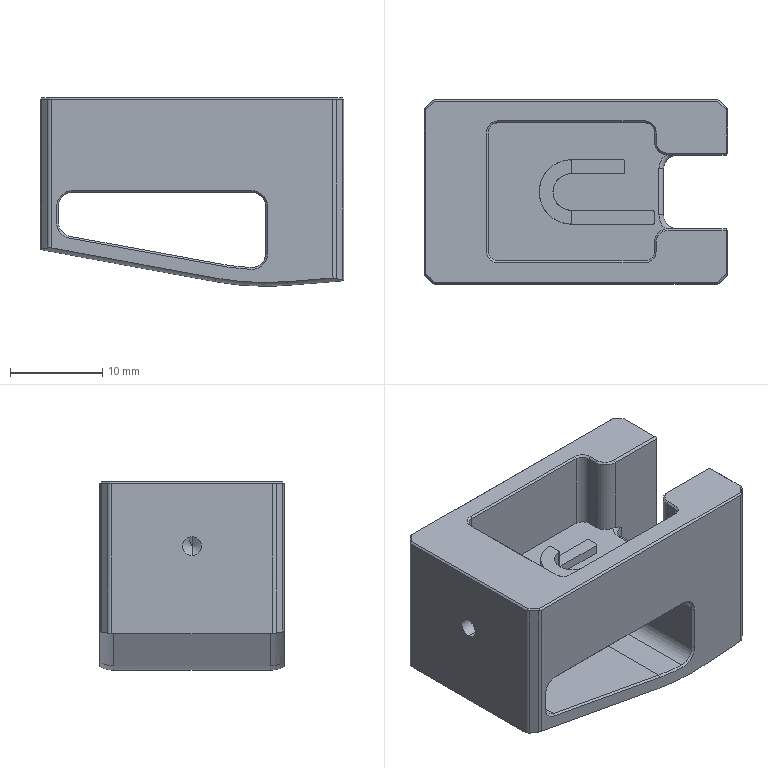NC program | NX | posted with a generic post | part box 33 x 20 x 20.478 mm
Lines 5322 to 6458 of 8500:
(CAVITY_MILL_COPY_COPY , TOOL : D2)
N10606 T17 M6
N10608 G54
N10610 G17 G0 G90 X-6.603 Y6.151 B0. C0. S9500 M3
N10612 G43 Z11. H17
N10614 Z1.351
N10616 G94 G1 Z-0.149 F1000.
N10618 G3 X-7.403 Y6.551 R1.
N10620 G1 X-8.5
N10622 X-8.554 Y6.554
N10624 X-8.551 Y6.5
N10626 Y5.403
N10628 G3 X-8.151 Y4.603 R1.
N10630 G1 Z1.351
N10632 G0 Z11.
N10634 X-6.552 Y6.1
N10636 Z1.203
N10638 G1 Z-0.297
N10640 G3 X-7.352 Y6.5 R1.
N10642 G1 X-8.5
N10644 Y5.352
N10646 G3 X-8.1 Y4.552 R1.
N10648 G1 Z1.203
N10650 G0 Z11.
N10652 X-6.552 Y6.1
N10654 Z1.054
N10656 G1 Z-0.446
N10658 G3 X-7.352 Y6.5 R1.
N10660 G1 X-8.5
N10662 Y5.352
N10664 G3 X-8.1 Y4.552 R1.
N10666 G1 Z1.054
N10668 G0 Z11.
N10670 X-6.552 Y6.1
N10672 Z0.905
N10674 G1 Z-0.595
N10676 G3 X-7.352 Y6.5 R1.
N10678 G1 X-8.5
N10680 Y5.352
N10682 G3 X-8.1 Y4.552 R1.
N10684 G1 Z0.905
N10686 G0 Z11.
N10688 X-6.552 Y6.1
N10690 Z0.756
N10692 G1 Z-0.744
N10694 G3 X-7.352 Y6.5 R1.
N10696 G1 X-8.5
N10698 Y5.352
N10700 G3 X-8.1 Y4.552 R1.
N10702 G1 Z0.756
N10704 G0 Z11.
N10706 X-6.552 Y6.1
N10708 Z0.608
N10710 G1 Z-0.892
N10712 G3 X-7.352 Y6.5 R1.
N10714 G1 X-8.5
N10716 Y5.352
N10718 G3 X-8.1 Y4.552 R1.
N10720 G1 Z0.608
N10722 G0 Z11.
N10724 X-6.552 Y6.1
N10726 Z0.459
N10728 G1 Z-1.041
N10730 G3 X-7.352 Y6.5 R1.
N10732 G1 X-8.5
N10734 Y5.352
N10736 G3 X-8.1 Y4.552 R1.
N10738 G1 Z0.459
N10740 G0 Z11.
N10742 X-6.552 Y6.1
N10744 Z0.31
N10746 G1 Z-1.19
N10748 G3 X-7.352 Y6.5 R1.
N10750 G1 X-8.5
N10752 Y5.352
N10754 G3 X-8.1 Y4.552 R1.
N10756 G1 Z0.31
N10758 G0 Z11.
N10760 X-6.552 Y6.1
N10762 Z0.162
N10764 G1 Z-1.338
N10766 G3 X-7.352 Y6.5 R1.
N10768 G1 X-8.5
N10770 Y5.352
N10772 G3 X-8.1 Y4.552 R1.
N10774 G1 Z0.162
N10776 G0 Z11.
N10778 X-6.552 Y6.1
N10780 Z0.013
N10782 G1 Z-1.487
N10784 G3 X-7.352 Y6.5 R1.
N10786 G1 X-8.5
N10788 Y5.352
N10790 G3 X-8.1 Y4.552 R1.
N10792 G1 Z0.013
N10794 G0 X-6.552 Y6.1 Z-0.136
N10796 G1 Z-1.636
N10798 G3 X-7.352 Y6.5 R1.
N10800 G1 X-8.5
N10802 Y5.352
N10804 G3 X-8.1 Y4.552 R1.
N10806 G1 Z-0.136
N10808 G0 X-6.552 Y6.1 Z-0.285
N10810 G1 Z-1.785
N10812 G3 X-7.352 Y6.5 R1.
N10814 G1 X-8.5
N10816 Y5.352
N10818 G3 X-8.1 Y4.552 R1.
N10820 G1 Z-0.285
N10822 G0 X-6.552 Y6.1 Z-0.433
N10824 G1 Z-1.933
N10826 G3 X-7.352 Y6.5 R1.
N10828 G1 X-8.5
N10830 Y5.352
N10832 G3 X-8.1 Y4.552 R1.
N10834 G1 Z-0.433
N10836 G0 X-6.552 Y6.1 Z-0.582
N10838 G1 Z-2.082
N10840 G3 X-7.352 Y6.5 R1.
N10842 G1 X-8.5
N10844 Y5.352
N10846 G3 X-8.1 Y4.552 R1.
N10848 G1 Z-0.582
N10850 G0 X-6.552 Y6.1 Z-0.731
N10852 G1 Z-2.231
N10854 G3 X-7.352 Y6.5 R1.
N10856 G1 X-8.5
N10858 Y5.352
N10860 G3 X-8.1 Y4.552 R1.
N10862 G1 Z-0.731
N10864 G0 X-6.552 Y6.1 Z-0.879
N10866 G1 Z-2.379
N10868 G3 X-7.352 Y6.5 R1.
N10870 G1 X-8.5
N10872 Y5.352
N10874 G3 X-8.1 Y4.552 R1.
N10876 G1 Z-0.879
N10878 G0 X-6.552 Y6.1 Z-1.028
N10880 G1 Z-2.528
N10882 G3 X-7.352 Y6.5 R1.
N10884 G1 X-8.5
N10886 Y5.352
N10888 G3 X-8.1 Y4.552 R1.
N10890 G1 Z-1.028
N10892 G0 X-6.552 Y6.1 Z-1.177
N10894 G1 Z-2.677
N10896 G3 X-7.352 Y6.5 R1.
N10898 G1 X-8.5
N10900 Y5.352
N10902 G3 X-8.1 Y4.552 R1.
N10904 G1 Z-1.177
N10906 G0 X-6.552 Y6.1 Z-1.326
N10908 G1 Z-2.826
N10910 G3 X-7.352 Y6.5 R1.
N10912 G1 X-8.5
N10914 Y5.352
N10916 G3 X-8.1 Y4.552 R1.
N10918 G1 Z-1.326
N10920 G0 X-6.552 Y6.1 Z-1.474
N10922 G1 Z-2.974
N10924 G3 X-7.352 Y6.5 R1.
N10926 G1 X-8.5
N10928 Y5.352
N10930 G3 X-8.1 Y4.552 R1.
N10932 G1 Z-1.474
N10934 G0 X-6.552 Y6.1 Z-1.623
N10936 G1 Z-3.123
N10938 G3 X-7.352 Y6.5 R1.
N10940 G1 X-8.5
N10942 Y5.352
N10944 G3 X-8.1 Y4.552 R1.
N10946 G1 Z-1.623
N10948 G0 X-6.552 Y6.1 Z-1.772
N10950 G1 Z-3.272
N10952 G3 X-7.352 Y6.5 R1.
N10954 G1 X-8.5
N10956 Y5.352
N10958 G3 X-8.1 Y4.552 R1.
N10960 G1 Z-1.772
N10962 G0 X-6.552 Y6.1 Z-1.921
N10964 G1 Z-3.421
N10966 G3 X-7.352 Y6.5 R1.
N10968 G1 X-8.5
N10970 Y5.352
N10972 G3 X-8.1 Y4.552 R1.
N10974 G1 Z-1.921
N10976 G0 X-6.552 Y6.1 Z-2.069
N10978 G1 Z-3.569
N10980 G3 X-7.352 Y6.5 R1.
N10982 G1 X-8.5
N10984 Y5.352
N10986 G3 X-8.1 Y4.552 R1.
N10988 G1 Z-2.069
N10990 G0 X-6.552 Y6.1 Z-2.218
N10992 G1 Z-3.718
N10994 G3 X-7.352 Y6.5 R1.
N10996 G1 X-8.5
N10998 Y5.352
N11000 G3 X-8.1 Y4.552 R1.
N11002 G1 Z-2.218
N11004 G0 X-6.552 Y6.1 Z-2.367
N11006 G1 Z-3.867
N11008 G3 X-7.352 Y6.5 R1.
N11010 G1 X-8.5
N11012 Y5.352
N11014 G3 X-8.1 Y4.552 R1.
N11016 G1 Z-2.367
N11018 G0 X-6.552 Y6.1 Z-2.515
N11020 G1 Z-4.015
N11022 G3 X-7.352 Y6.5 R1.
N11024 G1 X-8.5
N11026 Y5.352
N11028 G3 X-8.1 Y4.552 R1.
N11030 G1 Z-2.515
N11032 G0 X-6.552 Y6.1 Z-2.664
N11034 G1 Z-4.164
N11036 G3 X-7.352 Y6.5 R1.
N11038 G1 X-8.5
N11040 Y5.352
N11042 G3 X-8.1 Y4.552 R1.
N11044 G1 Z-2.664
N11046 G0 X-6.552 Y6.1 Z-2.813
N11048 G1 Z-4.313
N11050 G3 X-7.352 Y6.5 R1.
N11052 G1 X-8.5
N11054 Y5.352
N11056 G3 X-8.1 Y4.552 R1.
N11058 G1 Z-2.813
N11060 G0 X-6.552 Y6.1 Z-2.962
N11062 G1 Z-4.462
N11064 G3 X-7.352 Y6.5 R1.
N11066 G1 X-8.5
N11068 Y5.352
N11070 G3 X-8.1 Y4.552 R1.
N11072 G1 Z-2.962
N11074 G0 X-6.552 Y6.1 Z-3.11
N11076 G1 Z-4.61
N11078 G3 X-7.352 Y6.5 R1.
N11080 G1 X-8.5
N11082 Y5.352
N11084 G3 X-8.1 Y4.552 R1.
N11086 G1 Z-3.11
N11088 G0 X-6.552 Y6.1 Z-3.259
N11090 G1 Z-4.759
N11092 G3 X-7.352 Y6.5 R1.
N11094 G1 X-8.5
N11096 Y5.352
N11098 G3 X-8.1 Y4.552 R1.
N11100 G1 Z-3.259
N11102 G0 X-6.552 Y6.1 Z-3.408
N11104 G1 Z-4.908
N11106 G3 X-7.352 Y6.5 R1.
N11108 G1 X-8.5
N11110 Y5.352
N11112 G3 X-8.1 Y4.552 R1.
N11114 G1 Z-3.408
N11116 G0 X-6.552 Y6.1 Z-3.556
N11118 G1 Z-5.056
N11120 G3 X-7.352 Y6.5 R1.
N11122 G1 X-8.5
N11124 Y5.352
N11126 G3 X-8.1 Y4.552 R1.
N11128 G1 Z-3.556
N11130 G0 X-6.552 Y6.1 Z-3.705
N11132 G1 Z-5.205
N11134 G3 X-7.352 Y6.5 R1.
N11136 G1 X-8.5
N11138 Y5.352
N11140 G3 X-8.1 Y4.552 R1.
N11142 G1 Z-3.705
N11144 G0 X-6.552 Y6.1 Z-3.854
N11146 G1 Z-5.354
N11148 G3 X-7.352 Y6.5 R1.
N11150 G1 X-8.5
N11152 Y5.352
N11154 G3 X-8.1 Y4.552 R1.
N11156 G1 Z-3.854
N11158 G0 X-6.552 Y6.1 Z-4.003
N11160 G1 Z-5.503
N11162 G3 X-7.352 Y6.5 R1.
N11164 G1 X-8.5
N11166 Y5.352
N11168 G3 X-8.1 Y4.552 R1.
N11170 G1 Z-4.003
N11172 G0 X-6.552 Y6.1 Z-4.151
N11174 G1 Z-5.651
N11176 G3 X-7.352 Y6.5 R1.
N11178 G1 X-8.5
N11180 Y5.352
N11182 G3 X-8.1 Y4.552 R1.
N11184 G1 Z-4.151
N11186 G0 X-6.552 Y6.1 Z-4.3
N11188 G1 Z-5.8
N11190 G3 X-7.352 Y6.5 R1.
N11192 G1 X-8.5
N11194 Y5.352
N11196 G3 X-8.1 Y4.552 R1.
N11198 G1 Z-4.3
N11200 G0 X-6.552 Y6.1 Z-4.443
N11202 G1 Z-5.943
N11204 G3 X-7.352 Y6.5 R1.
N11206 G1 X-8.5
N11208 Y5.352
N11210 G3 X-8.1 Y4.552 R1.
N11212 G1 Z-4.443
N11214 G0 X-6.552 Y6.1 Z-4.586
N11216 G1 Z-6.086
N11218 G3 X-7.352 Y6.5 R1.
N11220 G1 X-8.5
N11222 Y5.352
N11224 G3 X-8.1 Y4.552 R1.
N11226 G1 Z-4.586
N11228 G0 X-6.552 Y6.1 Z-4.729
N11230 G1 Z-6.229
N11232 G3 X-7.352 Y6.5 R1.
N11234 G1 X-8.5
N11236 Y5.352
N11238 G3 X-8.1 Y4.552 R1.
N11240 G1 Z-4.729
N11242 G0 X-6.552 Y6.1 Z-4.871
N11244 G1 Z-6.371
N11246 G3 X-7.352 Y6.5 R1.
N11248 G1 X-8.5
N11250 Y5.352
N11252 G3 X-8.1 Y4.552 R1.
N11254 G1 Z-4.871
N11256 G0 X-6.552 Y6.1 Z-5.014
N11258 G1 Z-6.514
N11260 G3 X-7.352 Y6.5 R1.
N11262 G1 X-8.5
N11264 Y5.352
N11266 G3 X-8.1 Y4.552 R1.
N11268 G1 Z-5.014
N11270 G0 X-6.552 Y6.1 Z-5.157
N11272 G1 Z-6.657
N11274 G3 X-7.352 Y6.5 R1.
N11276 G1 X-8.5
N11278 Y5.352
N11280 G3 X-8.1 Y4.552 R1.
N11282 G1 Z-5.157
N11284 G0 X-6.552 Y6.1 Z-5.3
N11286 G1 Z-6.8
N11288 G3 X-7.352 Y6.5 R1.
N11290 G1 X-8.5
N11292 Y5.352
N11294 G3 X-8.1 Y4.552 R1.
N11296 G1 Z-5.3
N11298 G0 X-6.552 Y6.1 Z-5.443
N11300 G1 Z-6.943
N11302 G3 X-7.352 Y6.5 R1.
N11304 G1 X-8.5
N11306 Y5.352
N11308 G3 X-8.1 Y4.552 R1.
N11310 G1 Z-5.443
N11312 G0 X-6.552 Y6.1 Z-5.586
N11314 G1 Z-7.086
N11316 G3 X-7.352 Y6.5 R1.
N11318 G1 X-8.5
N11320 Y5.352
N11322 G3 X-8.1 Y4.552 R1.
N11324 G1 Z-5.586
N11326 G0 X-6.552 Y6.1 Z-5.729
N11328 G1 Z-7.229
N11330 G3 X-7.352 Y6.5 R1.
N11332 G1 X-8.5
N11334 Y5.352
N11336 G3 X-8.1 Y4.552 R1.
N11338 G1 Z-5.729
N11340 G0 X-6.552 Y6.1 Z-5.871
N11342 G1 Z-7.371
N11344 G3 X-7.352 Y6.5 R1.
N11346 G1 X-8.5
N11348 Y5.352
N11350 G3 X-8.1 Y4.552 R1.
N11352 G1 Z-5.871
N11354 G0 X-6.552 Y6.1 Z-6.014
N11356 G1 Z-7.514
N11358 G3 X-7.352 Y6.5 R1.
N11360 G1 X-8.5
N11362 Y5.352
N11364 G3 X-8.1 Y4.552 R1.
N11366 G1 Z-6.014
N11368 G0 X-6.552 Y6.1 Z-6.157
N11370 G1 Z-7.657
N11372 G3 X-7.352 Y6.5 R1.
N11374 G1 X-8.5
N11376 Y5.352
N11378 G3 X-8.1 Y4.552 R1.
N11380 G1 Z-6.157
N11382 G0 X-6.552 Y6.1 Z-6.3
N11384 G1 Z-7.8
N11386 G3 X-7.352 Y6.5 R1.
N11388 G1 X-8.5
N11390 Y5.352
N11392 G3 X-8.1 Y4.552 R1.
N11394 G1 Z-6.3
N11396 G0 X-6.552 Y6.1 Z-6.443
N11398 G1 Z-7.943
N11400 G3 X-7.352 Y6.5 R1.
N11402 G1 X-8.5
N11404 Y5.352
N11406 G3 X-8.1 Y4.552 R1.
N11408 G1 Z-6.443
N11410 G0 X-6.552 Y6.1 Z-6.586
N11412 G1 Z-8.086
N11414 G3 X-7.352 Y6.5 R1.
N11416 G1 X-8.5
N11418 Y5.352
N11420 G3 X-8.1 Y4.552 R1.
N11422 G1 Z-6.586
N11424 G0 X-6.552 Y6.1 Z-6.729
N11426 G1 Z-8.229
N11428 G3 X-7.352 Y6.5 R1.
N11430 G1 X-8.5
N11432 Y5.352
N11434 G3 X-8.1 Y4.552 R1.
N11436 G1 Z-6.729
N11438 G0 X-6.552 Y6.1 Z-6.871
N11440 G1 Z-8.371
N11442 G3 X-7.352 Y6.5 R1.
N11444 G1 X-8.5
N11446 Y5.352
N11448 G3 X-8.1 Y4.552 R1.
N11450 G1 Z-6.871
N11452 G0 X-6.552 Y6.1 Z-7.014
N11454 G1 Z-8.514
N11456 G3 X-7.352 Y6.5 R1.
N11458 G1 X-8.5
N11460 Y5.352
N11462 G3 X-8.1 Y4.552 R1.
N11464 G1 Z-7.014
N11466 G0 X-6.552 Y6.1 Z-7.157
N11468 G1 Z-8.657
N11470 G3 X-7.352 Y6.5 R1.
N11472 G1 X-8.5
N11474 Y5.352
N11476 G3 X-8.1 Y4.552 R1.
N11478 G1 Z-7.157
N11480 G0 X-6.552 Y6.1 Z-7.3
N11482 G1 Z-8.8
N11484 G3 X-7.352 Y6.5 R1.
N11486 G1 X-8.5
N11488 Y5.352
N11490 G3 X-8.1 Y4.552 R1.
N11492 G1 Z-7.3
N11494 G0 Z11.
N11496 X-8.151 Y-4.603
N11498 Z1.351
N11500 G1 Z-0.149
N11502 G3 X-8.551 Y-5.403 R1.
N11504 G1 Y-6.5
N11506 X-8.554 Y-6.554
N11508 X-8.5 Y-6.551
N11510 X-7.403
N11512 G3 X-6.603 Y-6.151 R1.
N11514 G1 Z1.351
N11516 G0 Z11.
N11518 X-8.1 Y-4.552
N11520 Z1.203
N11522 G1 Z-0.297
N11524 G3 X-8.5 Y-5.352 R1.
N11526 G1 Y-6.5
N11528 X-7.352
N11530 G3 X-6.552 Y-6.1 R1.
N11532 G1 Z1.203
N11534 G0 Z11.
N11536 X-8.1 Y-4.552
N11538 Z1.054
N11540 G1 Z-0.446
N11542 G3 X-8.5 Y-5.352 R1.
N11544 G1 Y-6.5
N11546 X-7.352
N11548 G3 X-6.552 Y-6.1 R1.
N11550 G1 Z1.054
N11552 G0 Z11.
N11554 X-8.1 Y-4.552
N11556 Z0.905
N11558 G1 Z-0.595
N11560 G3 X-8.5 Y-5.352 R1.
N11562 G1 Y-6.5
N11564 X-7.352
N11566 G3 X-6.552 Y-6.1 R1.
N11568 G1 Z0.905
N11570 G0 Z11.
N11572 X-8.1 Y-4.552
N11574 Z0.756
N11576 G1 Z-0.744
N11578 G3 X-8.5 Y-5.352 R1.
N11580 G1 Y-6.5
N11582 X-7.352
N11584 G3 X-6.552 Y-6.1 R1.
N11586 G1 Z0.756
N11588 G0 Z11.
N11590 X-8.1 Y-4.552
N11592 Z0.608
N11594 G1 Z-0.892
N11596 G3 X-8.5 Y-5.352 R1.
N11598 G1 Y-6.5
N11600 X-7.352
N11602 G3 X-6.552 Y-6.1 R1.
N11604 G1 Z0.608
N11606 G0 Z11.
N11608 X-8.1 Y-4.552
N11610 Z0.459
N11612 G1 Z-1.041
N11614 G3 X-8.5 Y-5.352 R1.
N11616 G1 Y-6.5
N11618 X-7.352
N11620 G3 X-6.552 Y-6.1 R1.
N11622 G1 Z0.459
N11624 G0 Z11.
N11626 X-8.1 Y-4.552
N11628 Z0.31
N11630 G1 Z-1.19
N11632 G3 X-8.5 Y-5.352 R1.
N11634 G1 Y-6.5
N11636 X-7.352
N11638 G3 X-6.552 Y-6.1 R1.
N11640 G1 Z0.31
N11642 G0 Z11.
N11644 X-8.1 Y-4.552
N11646 Z0.162
N11648 G1 Z-1.338
N11650 G3 X-8.5 Y-5.352 R1.
N11652 G1 Y-6.5
N11654 X-7.352
N11656 G3 X-6.552 Y-6.1 R1.
N11658 G1 Z0.162
N11660 G0 Z11.
N11662 X-8.1 Y-4.552
N11664 Z0.013
N11666 G1 Z-1.487
N11668 G3 X-8.5 Y-5.352 R1.
N11670 G1 Y-6.5
N11672 X-7.352
N11674 G3 X-6.552 Y-6.1 R1.
N11676 G1 Z0.013
N11678 G0 X-8.1 Y-4.552 Z-0.136
N11680 G1 Z-1.636
N11682 G3 X-8.5 Y-5.352 R1.
N11684 G1 Y-6.5
N11686 X-7.352
N11688 G3 X-6.552 Y-6.1 R1.
N11690 G1 Z-0.136
N11692 G0 X-8.1 Y-4.552 Z-0.285
N11694 G1 Z-1.785
N11696 G3 X-8.5 Y-5.352 R1.
N11698 G1 Y-6.5
N11700 X-7.352
N11702 G3 X-6.552 Y-6.1 R1.
N11704 G1 Z-0.285
N11706 G0 X-8.1 Y-4.552 Z-0.433
N11708 G1 Z-1.933
N11710 G3 X-8.5 Y-5.352 R1.
N11712 G1 Y-6.5
N11714 X-7.352
N11716 G3 X-6.552 Y-6.1 R1.
N11718 G1 Z-0.433
N11720 G0 X-8.1 Y-4.552 Z-0.582
N11722 G1 Z-2.082
N11724 G3 X-8.5 Y-5.352 R1.
N11726 G1 Y-6.5
N11728 X-7.352
N11730 G3 X-6.552 Y-6.1 R1.
N11732 G1 Z-0.582
N11734 G0 X-8.1 Y-4.552 Z-0.731
N11736 G1 Z-2.231
N11738 G3 X-8.5 Y-5.352 R1.
N11740 G1 Y-6.5
N11742 X-7.352
N11744 G3 X-6.552 Y-6.1 R1.
N11746 G1 Z-0.731
N11748 G0 X-8.1 Y-4.552 Z-0.879
N11750 G1 Z-2.379
N11752 G3 X-8.5 Y-5.352 R1.
N11754 G1 Y-6.5
N11756 X-7.352
N11758 G3 X-6.552 Y-6.1 R1.
N11760 G1 Z-0.879
N11762 G0 X-8.1 Y-4.552 Z-1.028
N11764 G1 Z-2.528
N11766 G3 X-8.5 Y-5.352 R1.
N11768 G1 Y-6.5
N11770 X-7.352
N11772 G3 X-6.552 Y-6.1 R1.
N11774 G1 Z-1.028
N11776 G0 X-8.1 Y-4.552 Z-1.177
N11778 G1 Z-2.677
N11780 G3 X-8.5 Y-5.352 R1.
N11782 G1 Y-6.5
N11784 X-7.352
N11786 G3 X-6.552 Y-6.1 R1.
N11788 G1 Z-1.177
N11790 G0 X-8.1 Y-4.552 Z-1.326
N11792 G1 Z-2.826
N11794 G3 X-8.5 Y-5.352 R1.
N11796 G1 Y-6.5
N11798 X-7.352
N11800 G3 X-6.552 Y-6.1 R1.
N11802 G1 Z-1.326
N11804 G0 X-8.1 Y-4.552 Z-1.474
N11806 G1 Z-2.974
N11808 G3 X-8.5 Y-5.352 R1.
N11810 G1 Y-6.5
N11812 X-7.352
N11814 G3 X-6.552 Y-6.1 R1.
N11816 G1 Z-1.474
N11818 G0 X-8.1 Y-4.552 Z-1.623
N11820 G1 Z-3.123
N11822 G3 X-8.5 Y-5.352 R1.
N11824 G1 Y-6.5
N11826 X-7.352
N11828 G3 X-6.552 Y-6.1 R1.
N11830 G1 Z-1.623
N11832 G0 X-8.1 Y-4.552 Z-1.772
N11834 G1 Z-3.272
N11836 G3 X-8.5 Y-5.352 R1.
N11838 G1 Y-6.5
N11840 X-7.352
N11842 G3 X-6.552 Y-6.1 R1.
N11844 G1 Z-1.772
N11846 G0 X-8.1 Y-4.552 Z-1.921
N11848 G1 Z-3.421
N11850 G3 X-8.5 Y-5.352 R1.
N11852 G1 Y-6.5
N11854 X-7.352
N11856 G3 X-6.552 Y-6.1 R1.
N11858 G1 Z-1.921
N11860 G0 X-8.1 Y-4.552 Z-2.069
N11862 G1 Z-3.569
N11864 G3 X-8.5 Y-5.352 R1.
N11866 G1 Y-6.5
N11868 X-7.352
N11870 G3 X-6.552 Y-6.1 R1.
N11872 G1 Z-2.069
N11874 G0 X-8.1 Y-4.552 Z-2.218
N11876 G1 Z-3.718
N11878 G3 X-8.5 Y-5.352 R1.
N11880 G1 Y-6.5
N11882 X-7.352
N11884 G3 X-6.552 Y-6.1 R1.
N11886 G1 Z-2.218
N11888 G0 X-8.1 Y-4.552 Z-2.367
N11890 G1 Z-3.867
N11892 G3 X-8.5 Y-5.352 R1.
N11894 G1 Y-6.5
N11896 X-7.352
N11898 G3 X-6.552 Y-6.1 R1.
N11900 G1 Z-2.367
N11902 G0 X-8.1 Y-4.552 Z-2.515
N11904 G1 Z-4.015
N11906 G3 X-8.5 Y-5.352 R1.
N11908 G1 Y-6.5
N11910 X-7.352
N11912 G3 X-6.552 Y-6.1 R1.
N11914 G1 Z-2.515
N11916 G0 X-8.1 Y-4.552 Z-2.664
N11918 G1 Z-4.164
N11920 G3 X-8.5 Y-5.352 R1.
N11922 G1 Y-6.5
N11924 X-7.352
N11926 G3 X-6.552 Y-6.1 R1.
N11928 G1 Z-2.664
N11930 G0 X-8.1 Y-4.552 Z-2.813
N11932 G1 Z-4.313
N11934 G3 X-8.5 Y-5.352 R1.
N11936 G1 Y-6.5
N11938 X-7.352
N11940 G3 X-6.552 Y-6.1 R1.
N11942 G1 Z-2.813
N11944 G0 X-8.1 Y-4.552 Z-2.962
N11946 G1 Z-4.462
N11948 G3 X-8.5 Y-5.352 R1.
N11950 G1 Y-6.5
N11952 X-7.352
N11954 G3 X-6.552 Y-6.1 R1.
N11956 G1 Z-2.962
N11958 G0 X-8.1 Y-4.552 Z-3.11
N11960 G1 Z-4.61
N11962 G3 X-8.5 Y-5.352 R1.
N11964 G1 Y-6.5
N11966 X-7.352
N11968 G3 X-6.552 Y-6.1 R1.
N11970 G1 Z-3.11
N11972 G0 X-8.1 Y-4.552 Z-3.259
N11974 G1 Z-4.759
N11976 G3 X-8.5 Y-5.352 R1.
N11978 G1 Y-6.5
N11980 X-7.352
N11982 G3 X-6.552 Y-6.1 R1.
N11984 G1 Z-3.259
N11986 G0 X-8.1 Y-4.552 Z-3.408
N11988 G1 Z-4.908
N11990 G3 X-8.5 Y-5.352 R1.
N11992 G1 Y-6.5
N11994 X-7.352
N11996 G3 X-6.552 Y-6.1 R1.
N11998 G1 Z-3.408
N12000 G0 X-8.1 Y-4.552 Z-3.556
N12002 G1 Z-5.056
N12004 G3 X-8.5 Y-5.352 R1.
N12006 G1 Y-6.5
N12008 X-7.352
N12010 G3 X-6.552 Y-6.1 R1.
N12012 G1 Z-3.556
N12014 G0 X-8.1 Y-4.552 Z-3.705
N12016 G1 Z-5.205
N12018 G3 X-8.5 Y-5.352 R1.
N12020 G1 Y-6.5
N12022 X-7.352
N12024 G3 X-6.552 Y-6.1 R1.
N12026 G1 Z-3.705
N12028 G0 X-8.1 Y-4.552 Z-3.854
N12030 G1 Z-5.354
N12032 G3 X-8.5 Y-5.352 R1.
N12034 G1 Y-6.5
N12036 X-7.352
N12038 G3 X-6.552 Y-6.1 R1.
N12040 G1 Z-3.854
N12042 G0 X-8.1 Y-4.552 Z-4.003
N12044 G1 Z-5.503
N12046 G3 X-8.5 Y-5.352 R1.
N12048 G1 Y-6.5
N12050 X-7.352
N12052 G3 X-6.552 Y-6.1 R1.
N12054 G1 Z-4.003
N12056 G0 X-8.1 Y-4.552 Z-4.151
N12058 G1 Z-5.651
N12060 G3 X-8.5 Y-5.352 R1.
N12062 G1 Y-6.5
N12064 X-7.352
N12066 G3 X-6.552 Y-6.1 R1.
N12068 G1 Z-4.151
N12070 G0 X-8.1 Y-4.552 Z-4.3
N12072 G1 Z-5.8
N12074 G3 X-8.5 Y-5.352 R1.
N12076 G1 Y-6.5
N12078 X-7.352
N12080 G3 X-6.552 Y-6.1 R1.
N12082 G1 Z-4.3
N12084 G0 X-8.1 Y-4.552 Z-4.443
N12086 G1 Z-5.943
N12088 G3 X-8.5 Y-5.352 R1.
N12090 G1 Y-6.5
N12092 X-7.352
N12094 G3 X-6.552 Y-6.1 R1.
N12096 G1 Z-4.443
N12098 G0 X-8.1 Y-4.552 Z-4.586
N12100 G1 Z-6.086
N12102 G3 X-8.5 Y-5.352 R1.
N12104 G1 Y-6.5
N12106 X-7.352
N12108 G3 X-6.552 Y-6.1 R1.
N12110 G1 Z-4.586
N12112 G0 X-8.1 Y-4.552 Z-4.729
N12114 G1 Z-6.229
N12116 G3 X-8.5 Y-5.352 R1.
N12118 G1 Y-6.5
N12120 X-7.352
N12122 G3 X-6.552 Y-6.1 R1.
N12124 G1 Z-4.729
N12126 G0 X-8.1 Y-4.552 Z-4.871
N12128 G1 Z-6.371
N12130 G3 X-8.5 Y-5.352 R1.
N12132 G1 Y-6.5
N12134 X-7.352
N12136 G3 X-6.552 Y-6.1 R1.
N12138 G1 Z-4.871
N12140 G0 X-8.1 Y-4.552 Z-5.014
N12142 G1 Z-6.514
N12144 G3 X-8.5 Y-5.352 R1.
N12146 G1 Y-6.5
N12148 X-7.352
N12150 G3 X-6.552 Y-6.1 R1.
N12152 G1 Z-5.014
N12154 G0 X-8.1 Y-4.552 Z-5.157
N12156 G1 Z-6.657
N12158 G3 X-8.5 Y-5.352 R1.
N12160 G1 Y-6.5
N12162 X-7.352
N12164 G3 X-6.552 Y-6.1 R1.
N12166 G1 Z-5.157
N12168 G0 X-8.1 Y-4.552 Z-5.3
N12170 G1 Z-6.8
N12172 G3 X-8.5 Y-5.352 R1.
N12174 G1 Y-6.5
N12176 X-7.352
N12178 G3 X-6.552 Y-6.1 R1.
N12180 G1 Z-5.3
N12182 G0 X-8.1 Y-4.552 Z-5.443
N12184 G1 Z-6.943
N12186 G3 X-8.5 Y-5.352 R1.
N12188 G1 Y-6.5
N12190 X-7.352
N12192 G3 X-6.552 Y-6.1 R1.
N12194 G1 Z-5.443
N12196 G0 X-8.1 Y-4.552 Z-5.586
N12198 G1 Z-7.086
N12200 G3 X-8.5 Y-5.352 R1.
N12202 G1 Y-6.5
N12204 X-7.352
N12206 G3 X-6.552 Y-6.1 R1.
N12208 G1 Z-5.586
N12210 G0 X-8.1 Y-4.552 Z-5.729
N12212 G1 Z-7.229
N12214 G3 X-8.5 Y-5.352 R1.
N12216 G1 Y-6.5
N12218 X-7.352
N12220 G3 X-6.552 Y-6.1 R1.
N12222 G1 Z-5.729
N12224 G0 X-8.1 Y-4.552 Z-5.871
N12226 G1 Z-7.371
N12228 G3 X-8.5 Y-5.352 R1.
N12230 G1 X-8.499 Y-6.5
N12232 X-7.352
N12234 G3 X-6.552 Y-6.1 R1.
N12236 G1 Z-5.871
N12238 G0 X-8.1 Y-4.552 Z-6.014
N12240 G1 Z-7.514
N12242 G3 X-8.5 Y-5.352 R1.
N12244 G1 X-8.499 Y-6.5
N12246 X-7.352
N12248 G3 X-6.552 Y-6.1 R1.
N12250 G1 Z-6.014
N12252 G0 X-8.1 Y-4.552 Z-6.157
N12254 G1 Z-7.657
N12256 G3 X-8.5 Y-5.352 R1.
N12258 G1 X-8.499 Y-6.5
N12260 X-7.352
N12262 G3 X-6.552 Y-6.1 R1.
N12264 G1 Z-6.157
N12266 G0 X-8.1 Y-4.552 Z-6.3
N12268 G1 Z-7.8
N12270 G3 X-8.5 Y-5.352 R1.
N12272 G1 X-8.499 Y-6.5
N12274 X-7.352
N12276 G3 X-6.552 Y-6.1 R1.
N12278 G1 Z-6.3
N12280 G0 X-8.1 Y-4.552 Z-6.443
N12282 G1 Z-7.943
N12284 G3 X-8.5 Y-5.352 R1.
N12286 G1 X-8.499 Y-6.5
N12288 X-7.352
N12290 G3 X-6.552 Y-6.1 R1.
N12292 G1 Z-6.443
N12294 G0 X-8.1 Y-4.552 Z-6.586
N12296 G1 Z-8.086
N12298 G3 X-8.5 Y-5.352 R1.
N12300 G1 X-8.499 Y-6.5
N12302 X-7.352
N12304 G3 X-6.552 Y-6.1 R1.
N12306 G1 Z-6.586
N12308 G0 X-8.1 Y-4.552 Z-6.729
N12310 G1 Z-8.229
N12312 G3 X-8.5 Y-5.352 R1.
N12314 G1 X-8.499 Y-6.5
N12316 X-7.352
N12318 G3 X-6.552 Y-6.1 R1.
N12320 G1 Z-6.729
N12322 G0 X-8.1 Y-4.552 Z-6.871
N12324 G1 Z-8.371
N12326 G3 X-8.5 Y-5.352 R1.
N12328 G1 X-8.499 Y-6.5
N12330 X-7.352
N12332 G3 X-6.552 Y-6.1 R1.
N12334 G1 Z-6.871
N12336 G0 X-8.1 Y-4.552 Z-7.014
N12338 G1 Z-8.514
N12340 G3 X-8.5 Y-5.352 R1.
N12342 G1 X-8.499 Y-6.5
N12344 X-7.352
N12346 G3 X-6.552 Y-6.1 R1.
N12348 G1 Z-7.014
N12350 G0 X-8.1 Y-4.552 Z-7.157
N12352 G1 Z-8.657
N12354 G3 X-8.5 Y-5.352 R1.
N12356 G1 X-8.499 Y-6.5
N12358 X-7.352
N12360 G3 X-6.552 Y-6.1 R1.
N12362 G1 Z-7.157
N12364 G0 X-8.1 Y-4.552 Z-7.3
N12366 G1 Z-8.8
N12368 G3 X-8.5 Y-5.352 R1.
N12370 G1 X-8.498 Y-6.5
N12372 X-7.352
N12374 G3 X-6.552 Y-6.1 R1.
N12376 G1 Z-7.3
N12378 G0 Z11.
N12380 X5.566 Y0.624
N12382 Z-6.443
N12384 G1 Z-7.943
N12386 X5.04 Y0.866
N12388 G3 X4.54 Y0. R1.
N12390 G1 X3.64
N12392 X3.643 Y0.1
N12394 X-0.505
N12396 X-0.567 Y0.112
N12398 X-0.586 Y0.051
N12400 G3 X-0.5 Y-0.1 R0.1
N12402 G1 X3.643
N12404 X3.64 Y0.
N12406 X4.54
N12408 X4.541 Y0.038
N12410 G2 X4.914 Y0.528 R0.56
N12412 G3 X5.248 Y1.009 R0.5
N12414 G1 X5.1 Y1.
N12416 X-0.553
N12418 X-0.591 Y0.996
N12420 G3 X-0.5 Y-1. R1.
N12422 G1 X5.248
N12424 G3 X4.914 Y-0.528 R0.5
N12426 G2 X4.54 Y0. R0.56
N12428 X5.04 Y0.866 R1.
N12430 G1 X5.566 Y0.624
N12432 Z-6.443
N12434 G0 Z-6.586
N12436 G1 Z-8.086
N12438 X5.04 Y0.866
N12440 G3 X4.54 Y0. R1.
N12442 G1 X3.64
N12444 X3.643 Y0.1
N12446 X-0.505
N12448 X-0.567 Y0.112
N12450 X-0.586 Y0.051
N12452 G3 X-0.5 Y-0.1 R0.1
N12454 G1 X3.643
N12456 X3.64 Y0.
N12458 X4.54
N12460 X4.541 Y0.038
N12462 G2 X4.914 Y0.528 R0.56
N12464 G3 X5.248 Y1.009 R0.5
N12466 G1 X5.1 Y1.
N12468 X-0.553
N12470 X-0.591 Y0.996
N12472 G3 X-0.5 Y-1. R1.
N12474 G1 X5.248
N12476 G3 X4.914 Y-0.528 R0.5
N12478 G2 X4.54 Y0. R0.56
N12480 X5.04 Y0.866 R1.
N12482 G1 X5.566 Y0.624
N12484 Z-6.586
N12486 G0 Z-6.729
N12488 G1 Z-8.229
N12490 X5.04 Y0.866
N12492 G3 X4.54 Y0. R1.
N12494 G1 X3.64
N12496 X3.643 Y0.1
N12498 X-0.505
N12500 X-0.567 Y0.112
N12502 X-0.586 Y0.051
N12504 G3 X-0.5 Y-0.1 R0.1
N12506 G1 X3.643
N12508 X3.64 Y0.
N12510 X4.54
N12512 X4.541 Y0.038
N12514 G2 X4.914 Y0.528 R0.56
N12516 G3 X5.248 Y1.009 R0.5
N12518 G1 X5.1 Y1.
N12520 X-0.553
N12522 X-0.591 Y0.996
N12524 G3 X-0.5 Y-1. R1.
N12526 G1 X5.248
N12528 G3 X4.914 Y-0.528 R0.5
N12530 G2 X4.54 Y0. R0.56
N12532 X5.04 Y0.866 R1.
N12534 G1 X5.566 Y0.624
N12536 Z-6.729
N12538 G0 Z-6.871
N12540 G1 Z-8.371
N12542 X5.04 Y0.866
N12544 G3 X4.54 Y0. R1.
N12546 G1 X3.64
N12548 X3.643 Y0.1
N12550 X-0.505
N12552 X-0.567 Y0.112
N12554 X-0.586 Y0.051
N12556 G3 X-0.5 Y-0.1 R0.1
N12558 G1 X3.643
N12560 X3.64 Y0.
N12562 X4.54
N12564 X4.541 Y0.038
N12566 G2 X4.914 Y0.528 R0.56
N12568 G3 X5.248 Y1.009 R0.5
N12570 G1 X5.1 Y1.
N12572 X-0.553
N12574 X-0.591 Y0.996
N12576 G3 X-0.5 Y-1. R1.
N12578 G1 X5.248
N12580 G3 X4.914 Y-0.528 R0.5
N12582 G2 X4.54 Y0. R0.56
N12584 X5.04 Y0.866 R1.
N12586 G1 X5.566 Y0.624
N12588 Z-6.871
N12590 G0 Z-7.014
N12592 G1 Z-8.514
N12594 X5.04 Y0.866
N12596 G3 X4.54 Y0. R1.
N12598 G1 X3.64
N12600 X3.643 Y0.1
N12602 X-0.505
N12604 X-0.567 Y0.112
N12606 X-0.586 Y0.051
N12608 G3 X-0.5 Y-0.1 R0.1
N12610 G1 X3.643
N12612 X3.64 Y0.
N12614 X4.54
N12616 X4.541 Y0.038
N12618 G2 X4.914 Y0.528 R0.56
N12620 G3 X5.248 Y1.009 R0.5
N12622 G1 X5.1 Y1.
N12624 X-0.553
N12626 X-0.591 Y0.996
N12628 G3 X-0.5 Y-1. R1.
N12630 G1 X5.248
N12632 G3 X4.914 Y-0.528 R0.5
N12634 G2 X4.54 Y0. R0.56
N12636 X5.04 Y0.866 R1.
N12638 G1 X5.566 Y0.624
N12640 Z-7.014
N12642 G0 Z-7.157
N12644 G1 Z-8.657
N12646 X5.04 Y0.866
N12648 G3 X4.54 Y0. R1.
N12650 G1 X3.64
N12652 X3.643 Y0.1
N12654 X-0.505
N12656 X-0.567 Y0.112
N12658 X-0.586 Y0.051
N12660 G3 X-0.5 Y-0.1 R0.1
N12662 G1 X3.643
N12664 X3.64 Y0.
N12666 X4.54
N12668 X4.541 Y0.038
N12670 G2 X4.914 Y0.528 R0.56
N12672 G3 X5.248 Y1.009 R0.5
N12674 G1 X5.1 Y1.
N12676 X-0.553
N12678 X-0.591 Y0.996
N12680 G3 X-0.5 Y-1. R1.
N12682 G1 X5.248
N12684 G3 X4.914 Y-0.528 R0.5
N12686 G2 X4.54 Y0. R0.56
N12688 X5.04 Y0.866 R1.
N12690 G1 X5.566 Y0.624
N12692 Z-7.157
N12694 G0 Z-7.3
N12696 G1 Z-8.8
N12698 X5.04 Y0.866
N12700 G3 X4.54 Y0. R1.
N12702 G1 X3.64
N12704 X3.643 Y0.1
N12706 X-0.505
N12708 X-0.567 Y0.112
N12710 X-0.586 Y0.051
N12712 G3 X-0.5 Y-0.1 R0.1
N12714 G1 X3.643
N12716 X3.64 Y0.
N12718 X4.54
N12720 X4.541 Y0.038
N12722 G2 X4.914 Y0.528 R0.56
N12724 G3 X5.248 Y1.009 R0.5
N12726 G1 X5.1 Y1.
N12728 X-0.553
N12730 X-0.591 Y0.996
N12732 G3 X-0.5 Y-1. R1.
N12734 G1 X5.248
N12736 G3 X4.914 Y-0.528 R0.5
N12738 G2 X4.54 Y0. R0.56
N12740 X5.04 Y0.866 R1.
N12742 G1 X5.566 Y0.624
N12744 Z-7.3
N12746 G0 Z11.
N12748 X5.603 Y-6.151
N12750 Z1.351
N12752 G1 Z-0.149
N12754 G3 X6.403 Y-6.551 R1.
N12756 G1 X7.5
N12758 X7.554 Y-6.554
N12760 X7.551 Y-6.5
N12762 Y-5.5
N12764 X7.553 Y-5.403
N12766 G3 X7.275 Y-4.67 R1.
N12768 G1 Z1.351
N12770 G0 Z11.
N12772 X5.552 Y-6.1
N12774 Z1.203
N12776 G1 Z-0.297
N12778 G3 X6.352 Y-6.5 R1.
N12780 G1 X7.5
N12782 Y-5.5
N12784 X7.504 Y-5.351
N12786 G3 X7.239 Y-4.612 R1.
N12788 G1 Z1.203
N12790 G0 Z11.
N12792 X5.552 Y-6.1
N12794 Z1.054
N12796 G1 Z-0.446
N12798 G3 X6.352 Y-6.5 R1.
N12800 G1 X7.5
N12802 Y-5.5
N12804 X7.504 Y-5.351
N12806 G3 X7.239 Y-4.612 R1.
N12808 G1 Z1.054
N12810 G0 Z11.
N12812 X5.551 Y-6.1
N12814 Z0.905
N12816 G1 Z-0.595
N12818 G3 X6.351 Y-6.5 R1.
N12820 G1 X7.5
N12822 Y-5.5
N12824 X7.504 Y-5.351
N12826 G3 X7.239 Y-4.612 R1.
N12828 G1 Z0.905
N12830 G0 Z11.
N12832 X5.551 Y-6.1
N12834 Z0.756
N12836 G1 Z-0.744
N12838 G3 X6.351 Y-6.5 R1.
N12840 G1 X7.5
N12842 Y-5.5
N12844 X7.504 Y-5.351
N12846 G3 X7.239 Y-4.612 R1.
N12848 G1 Z0.756
N12850 G0 Z11.
N12852 X5.551 Y-6.1
N12854 Z0.608
N12856 G1 Z-0.892
N12858 G3 X6.351 Y-6.5 R1.
N12860 G1 X7.5
N12862 Y-5.5
N12864 X7.504 Y-5.351
N12866 G3 X7.239 Y-4.612 R1.
N12868 G1 Z0.608
N12870 G0 Z11.
N12872 X5.551 Y-6.1